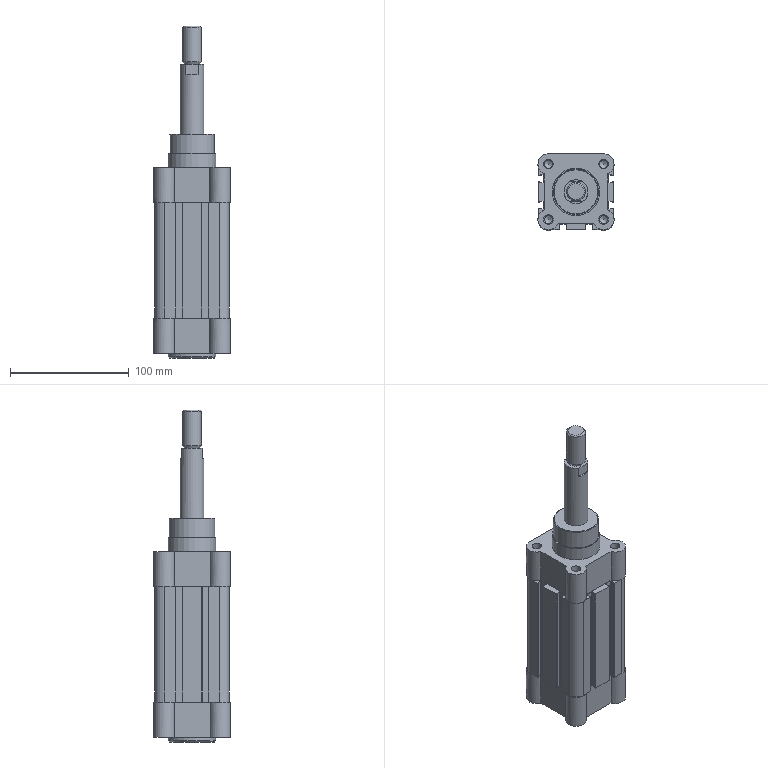Part | STEP file | 163371 DNC-50-50-PPV-A | 2 solids | 197 faces | box 64 x 64 x 279 mm | volume 523185 mm3 | plane 89 | cylinder 86 | cone 22 | commonest cylinder face diameters 0.6 x24 0.8 x24 17.5 x12 6.647 x8 8 x8 11.445 x2